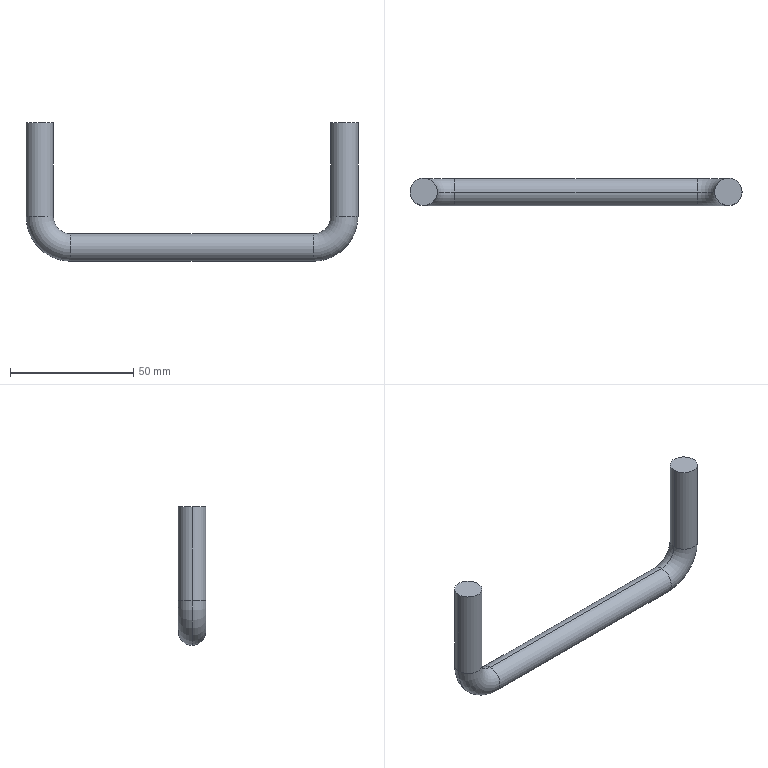Part | NX | features BREP 1 | 1 solid | 12 faces | box 134.938 x 11.113 x 56.356 mm | volume 20806 mm3 | cylinder 6 | torus 4 | plane 2 | commonest cylinder face diameters 11.113 x6
STEP:
#1=CARTESIAN_POINT('',(-56.356,0.,0.));
#2=VERTEX_POINT('',#1);
#3=CARTESIAN_POINT('',(-67.469,0.,0.));
#4=VERTEX_POINT('',#3);
#5=CARTESIAN_POINT('',(-61.913,0.,0.));
#6=DIRECTION('',(0.,0.,-1.));
#7=DIRECTION('',(1.,0.,0.));
#8=AXIS2_PLACEMENT_3D('',#5,#6,#7);
#9=CIRCLE('',#8,5.556);
#10=EDGE_CURVE('',#2,#4,#9,.T.);
#11=ORIENTED_EDGE('',*,*,#10,.F.);
#12=CARTESIAN_POINT('',(-61.913,0.,0.));
#13=DIRECTION('',(0.,0.,-1.));
#14=DIRECTION('',(-1.,0.,0.));
#15=AXIS2_PLACEMENT_3D('',#12,#13,#14);
#16=CIRCLE('',#15,5.556);
#17=EDGE_CURVE('',#4,#2,#16,.T.);
#18=ORIENTED_EDGE('',*,*,#17,.F.);
#19=EDGE_LOOP('',(#11,#18));
#20=FACE_BOUND('',#19,.T.);
#21=CARTESIAN_POINT('',(-61.913,0.,0.));
#22=DIRECTION('',(0.,0.,-1.));
#23=DIRECTION('',(0.,-1.,0.));
#24=AXIS2_PLACEMENT_3D('',#21,#22,#23);
#25=PLANE('',#24);
#26=ADVANCED_FACE('',(#20),#25,.F.);
#27=CARTESIAN_POINT('',(-56.356,0.,-38.1));
#28=VERTEX_POINT('',#27);
#29=CARTESIAN_POINT('',(-56.356,0.,0.));
#30=DIRECTION('',(0.,0.,-1.));
#31=VECTOR('',#30,1000.);
#32=LINE('',#29,#31);
#33=EDGE_CURVE('',#28,#2,#32,.F.);
#34=ORIENTED_EDGE('',*,*,#33,.F.);
#35=CARTESIAN_POINT('',(-67.469,0.,-38.1));
#36=VERTEX_POINT('',#35);
#37=CARTESIAN_POINT('',(-61.913,0.,-38.1));
#38=DIRECTION('',(0.,0.,-1.));
#39=DIRECTION('',(-1.,0.,0.));
#40=AXIS2_PLACEMENT_3D('',#37,#38,#39);
#41=CIRCLE('',#40,5.556);
#42=EDGE_CURVE('',#36,#28,#41,.T.);
#43=ORIENTED_EDGE('',*,*,#42,.F.);
#44=CARTESIAN_POINT('',(-67.469,0.,0.));
#45=DIRECTION('',(0.,0.,-1.));
#46=VECTOR('',#45,1000.);
#47=LINE('',#44,#46);
#48=EDGE_CURVE('',#36,#4,#47,.F.);
#49=ORIENTED_EDGE('',*,*,#48,.T.);
#50=ORIENTED_EDGE('',*,*,#17,.T.);
#51=EDGE_LOOP('',(#34,#43,#49,#50));
#52=FACE_BOUND('',#51,.T.);
#53=CARTESIAN_POINT('',(-61.913,0.,0.));
#54=DIRECTION('',(0.,0.,-1.));
#55=DIRECTION('',(-1.,0.,0.));
#56=AXIS2_PLACEMENT_3D('',#53,#54,#55);
#57=CYLINDRICAL_SURFACE('',#56,5.556);
#58=ADVANCED_FACE('',(#52),#57,.T.);
#59=ORIENTED_EDGE('',*,*,#48,.F.);
#60=CARTESIAN_POINT('',(-61.913,0.,-38.1));
#61=DIRECTION('',(0.,0.,-1.));
#62=DIRECTION('',(1.,0.,0.));
#63=AXIS2_PLACEMENT_3D('',#60,#61,#62);
#64=CIRCLE('',#63,5.556);
#65=EDGE_CURVE('',#28,#36,#64,.T.);
#66=ORIENTED_EDGE('',*,*,#65,.F.);
#67=ORIENTED_EDGE('',*,*,#33,.T.);
#68=ORIENTED_EDGE('',*,*,#10,.T.);
#69=EDGE_LOOP('',(#59,#66,#67,#68));
#70=FACE_BOUND('',#69,.T.);
#71=CARTESIAN_POINT('',(-61.913,0.,0.));
#72=DIRECTION('',(0.,0.,-1.));
#73=DIRECTION('',(-1.,0.,0.));
#74=AXIS2_PLACEMENT_3D('',#71,#72,#73);
#75=CYLINDRICAL_SURFACE('',#74,5.556);
#76=ADVANCED_FACE('',(#70),#75,.T.);
#77=CARTESIAN_POINT('',(-49.212,0.,-56.356));
#78=VERTEX_POINT('',#77);
#79=CARTESIAN_POINT('',(-49.212,0.,-38.1));
#80=DIRECTION('',(0.,-1.,0.));
#81=DIRECTION('',(-1.,0.,0.));
#82=AXIS2_PLACEMENT_3D('',#79,#80,#81);
#83=CIRCLE('',#82,18.256);
#84=EDGE_CURVE('',#36,#78,#83,.T.);
#85=ORIENTED_EDGE('',*,*,#84,.T.);
#86=CARTESIAN_POINT('',(-49.212,0.,-45.244));
#87=VERTEX_POINT('',#86);
#88=CARTESIAN_POINT('',(-49.212,0.,-50.8));
#89=DIRECTION('',(1.,0.,0.));
#90=DIRECTION('',(0.,0.,1.));
#91=AXIS2_PLACEMENT_3D('',#88,#89,#90);
#92=CIRCLE('',#91,5.556);
#93=EDGE_CURVE('',#87,#78,#92,.T.);
#94=ORIENTED_EDGE('',*,*,#93,.F.);
#95=CARTESIAN_POINT('',(-49.212,0.,-38.1));
#96=DIRECTION('',(0.,-1.,0.));
#97=DIRECTION('',(-1.,0.,0.));
#98=AXIS2_PLACEMENT_3D('',#95,#96,#97);
#99=CIRCLE('',#98,7.144);
#100=EDGE_CURVE('',#28,#87,#99,.T.);
#101=ORIENTED_EDGE('',*,*,#100,.F.);
#102=ORIENTED_EDGE('',*,*,#65,.T.);
#103=EDGE_LOOP('',(#85,#94,#101,#102));
#104=FACE_BOUND('',#103,.T.);
#105=CARTESIAN_POINT('',(-49.212,0.,-38.1));
#106=DIRECTION('',(0.,-1.,0.));
#107=DIRECTION('',(1.,0.,0.));
#108=AXIS2_PLACEMENT_3D('',#105,#106,#107);
#109=TOROIDAL_SURFACE('',#108,12.7,5.556);
#110=ADVANCED_FACE('',(#104),#109,.T.);
#111=ORIENTED_EDGE('',*,*,#100,.T.);
#112=CARTESIAN_POINT('',(-49.212,0.,-50.8));
#113=DIRECTION('',(1.,0.,0.));
#114=DIRECTION('',(0.,0.,-1.));
#115=AXIS2_PLACEMENT_3D('',#112,#113,#114);
#116=CIRCLE('',#115,5.556);
#117=EDGE_CURVE('',#78,#87,#116,.T.);
#118=ORIENTED_EDGE('',*,*,#117,.F.);
#119=ORIENTED_EDGE('',*,*,#84,.F.);
#120=ORIENTED_EDGE('',*,*,#42,.T.);
#121=EDGE_LOOP('',(#111,#118,#119,#120));
#122=FACE_BOUND('',#121,.T.);
#123=CARTESIAN_POINT('',(-49.212,0.,-38.1));
#124=DIRECTION('',(0.,-1.,0.));
#125=DIRECTION('',(1.,0.,0.));
#126=AXIS2_PLACEMENT_3D('',#123,#124,#125);
#127=TOROIDAL_SURFACE('',#126,12.7,5.556);
#128=ADVANCED_FACE('',(#122),#127,.T.);
#129=CARTESIAN_POINT('',(49.212,0.,-45.244));
#130=VERTEX_POINT('',#129);
#131=CARTESIAN_POINT('',(-49.212,0.,-45.244));
#132=DIRECTION('',(1.,0.,0.));
#133=VECTOR('',#132,1000.);
#134=LINE('',#131,#133);
#135=EDGE_CURVE('',#130,#87,#134,.F.);
#136=ORIENTED_EDGE('',*,*,#135,.F.);
#137=CARTESIAN_POINT('',(49.212,0.,-56.356));
#138=VERTEX_POINT('',#137);
#139=CARTESIAN_POINT('',(49.212,0.,-50.8));
#140=DIRECTION('',(1.,0.,0.));
#141=DIRECTION('',(0.,0.,-1.));
#142=AXIS2_PLACEMENT_3D('',#139,#140,#141);
#143=CIRCLE('',#142,5.556);
#144=EDGE_CURVE('',#138,#130,#143,.T.);
#145=ORIENTED_EDGE('',*,*,#144,.F.);
#146=CARTESIAN_POINT('',(-49.212,0.,-56.356));
#147=DIRECTION('',(1.,0.,0.));
#148=VECTOR('',#147,1000.);
#149=LINE('',#146,#148);
#150=EDGE_CURVE('',#138,#78,#149,.F.);
#151=ORIENTED_EDGE('',*,*,#150,.T.);
#152=ORIENTED_EDGE('',*,*,#117,.T.);
#153=EDGE_LOOP('',(#136,#145,#151,#152));
#154=FACE_BOUND('',#153,.T.);
#155=CARTESIAN_POINT('',(-49.212,0.,-50.8));
#156=DIRECTION('',(1.,0.,0.));
#157=DIRECTION('',(0.,0.,-1.));
#158=AXIS2_PLACEMENT_3D('',#155,#156,#157);
#159=CYLINDRICAL_SURFACE('',#158,5.556);
#160=ADVANCED_FACE('',(#154),#159,.T.);
#161=ORIENTED_EDGE('',*,*,#150,.F.);
#162=CARTESIAN_POINT('',(49.212,0.,-50.8));
#163=DIRECTION('',(1.,0.,0.));
#164=DIRECTION('',(0.,0.,1.));
#165=AXIS2_PLACEMENT_3D('',#162,#163,#164);
#166=CIRCLE('',#165,5.556);
#167=EDGE_CURVE('',#130,#138,#166,.T.);
#168=ORIENTED_EDGE('',*,*,#167,.F.);
#169=ORIENTED_EDGE('',*,*,#135,.T.);
#170=ORIENTED_EDGE('',*,*,#93,.T.);
#171=EDGE_LOOP('',(#161,#168,#169,#170));
#172=FACE_BOUND('',#171,.T.);
#173=CARTESIAN_POINT('',(-49.212,0.,-50.8));
#174=DIRECTION('',(1.,0.,0.));
#175=DIRECTION('',(0.,0.,-1.));
#176=AXIS2_PLACEMENT_3D('',#173,#174,#175);
#177=CYLINDRICAL_SURFACE('',#176,5.556);
#178=ADVANCED_FACE('',(#172),#177,.T.);
#179=CARTESIAN_POINT('',(67.469,0.,-38.1));
#180=VERTEX_POINT('',#179);
#181=CARTESIAN_POINT('',(49.212,0.,-38.1));
#182=DIRECTION('',(0.,-1.,0.));
#183=DIRECTION('',(0.,0.,-1.));
#184=AXIS2_PLACEMENT_3D('',#181,#182,#183);
#185=CIRCLE('',#184,18.256);
#186=EDGE_CURVE('',#138,#180,#185,.T.);
#187=ORIENTED_EDGE('',*,*,#186,.T.);
#188=CARTESIAN_POINT('',(56.356,0.,-38.1));
#189=VERTEX_POINT('',#188);
#190=CARTESIAN_POINT('',(61.913,0.,-38.1));
#191=DIRECTION('',(0.,0.,1.));
#192=DIRECTION('',(-1.,0.,0.));
#193=AXIS2_PLACEMENT_3D('',#190,#191,#192);
#194=CIRCLE('',#193,5.556);
#195=EDGE_CURVE('',#189,#180,#194,.T.);
#196=ORIENTED_EDGE('',*,*,#195,.F.);
#197=CARTESIAN_POINT('',(49.212,0.,-38.1));
#198=DIRECTION('',(0.,-1.,0.));
#199=DIRECTION('',(0.,0.,-1.));
#200=AXIS2_PLACEMENT_3D('',#197,#198,#199);
#201=CIRCLE('',#200,7.144);
#202=EDGE_CURVE('',#130,#189,#201,.T.);
#203=ORIENTED_EDGE('',*,*,#202,.F.);
#204=ORIENTED_EDGE('',*,*,#167,.T.);
#205=EDGE_LOOP('',(#187,#196,#203,#204));
#206=FACE_BOUND('',#205,.T.);
#207=CARTESIAN_POINT('',(49.212,0.,-38.1));
#208=DIRECTION('',(0.,-1.,0.));
#209=DIRECTION('',(0.,0.,1.));
#210=AXIS2_PLACEMENT_3D('',#207,#208,#209);
#211=TOROIDAL_SURFACE('',#210,12.7,5.556);
#212=ADVANCED_FACE('',(#206),#211,.T.);
#213=ORIENTED_EDGE('',*,*,#202,.T.);
#214=CARTESIAN_POINT('',(61.913,0.,-38.1));
#215=DIRECTION('',(0.,0.,1.));
#216=DIRECTION('',(1.,0.,0.));
#217=AXIS2_PLACEMENT_3D('',#214,#215,#216);
#218=CIRCLE('',#217,5.556);
#219=EDGE_CURVE('',#180,#189,#218,.T.);
#220=ORIENTED_EDGE('',*,*,#219,.F.);
#221=ORIENTED_EDGE('',*,*,#186,.F.);
#222=ORIENTED_EDGE('',*,*,#144,.T.);
#223=EDGE_LOOP('',(#213,#220,#221,#222));
#224=FACE_BOUND('',#223,.T.);
#225=CARTESIAN_POINT('',(49.212,0.,-38.1));
#226=DIRECTION('',(0.,-1.,0.));
#227=DIRECTION('',(0.,0.,1.));
#228=AXIS2_PLACEMENT_3D('',#225,#226,#227);
#229=TOROIDAL_SURFACE('',#228,12.7,5.556);
#230=ADVANCED_FACE('',(#224),#229,.T.);
#231=CARTESIAN_POINT('',(56.356,0.,0.));
#232=VERTEX_POINT('',#231);
#233=CARTESIAN_POINT('',(56.356,0.,-38.1));
#234=DIRECTION('',(0.,0.,1.));
#235=VECTOR('',#234,1000.);
#236=LINE('',#233,#235);
#237=EDGE_CURVE('',#189,#232,#236,.T.);
#238=ORIENTED_EDGE('',*,*,#237,.T.);
#239=CARTESIAN_POINT('',(67.469,0.,0.));
#240=VERTEX_POINT('',#239);
#241=CARTESIAN_POINT('',(61.913,0.,0.));
#242=DIRECTION('',(0.,0.,1.));
#243=DIRECTION('',(1.,0.,0.));
#244=AXIS2_PLACEMENT_3D('',#241,#242,#243);
#245=CIRCLE('',#244,5.556);
#246=EDGE_CURVE('',#240,#232,#245,.T.);
#247=ORIENTED_EDGE('',*,*,#246,.F.);
#248=CARTESIAN_POINT('',(67.469,0.,-38.1));
#249=DIRECTION('',(0.,0.,1.));
#250=VECTOR('',#249,1000.);
#251=LINE('',#248,#250);
#252=EDGE_CURVE('',#180,#240,#251,.T.);
#253=ORIENTED_EDGE('',*,*,#252,.F.);
#254=ORIENTED_EDGE('',*,*,#219,.T.);
#255=EDGE_LOOP('',(#238,#247,#253,#254));
#256=FACE_BOUND('',#255,.T.);
#257=CARTESIAN_POINT('',(61.913,0.,-38.1));
#258=DIRECTION('',(0.,0.,1.));
#259=DIRECTION('',(1.,0.,0.));
#260=AXIS2_PLACEMENT_3D('',#257,#258,#259);
#261=CYLINDRICAL_SURFACE('',#260,5.556);
#262=ADVANCED_FACE('',(#256),#261,.T.);
#263=ORIENTED_EDGE('',*,*,#252,.T.);
#264=CARTESIAN_POINT('',(61.913,0.,0.));
#265=DIRECTION('',(0.,0.,1.));
#266=DIRECTION('',(-1.,0.,0.));
#267=AXIS2_PLACEMENT_3D('',#264,#265,#266);
#268=CIRCLE('',#267,5.556);
#269=EDGE_CURVE('',#232,#240,#268,.T.);
#270=ORIENTED_EDGE('',*,*,#269,.F.);
#271=ORIENTED_EDGE('',*,*,#237,.F.);
#272=ORIENTED_EDGE('',*,*,#195,.T.);
#273=EDGE_LOOP('',(#263,#270,#271,#272));
#274=FACE_BOUND('',#273,.T.);
#275=CARTESIAN_POINT('',(61.913,0.,-38.1));
#276=DIRECTION('',(0.,0.,1.));
#277=DIRECTION('',(1.,0.,0.));
#278=AXIS2_PLACEMENT_3D('',#275,#276,#277);
#279=CYLINDRICAL_SURFACE('',#278,5.556);
#280=ADVANCED_FACE('',(#274),#279,.T.);
#281=ORIENTED_EDGE('',*,*,#269,.T.);
#282=ORIENTED_EDGE('',*,*,#246,.T.);
#283=EDGE_LOOP('',(#281,#282));
#284=FACE_BOUND('',#283,.T.);
#285=CARTESIAN_POINT('',(61.913,0.,0.));
#286=DIRECTION('',(0.,0.,1.));
#287=DIRECTION('',(1.,0.,0.));
#288=AXIS2_PLACEMENT_3D('',#285,#286,#287);
#289=PLANE('',#288);
#290=ADVANCED_FACE('',(#284),#289,.T.);
#291=CLOSED_SHELL('',(#26,#58,#76,#110,#128,#160,#178,#212,#230,#262,#280,#290));
#292=MANIFOLD_SOLID_BREP('',#291);
#293=(LENGTH_UNIT()NAMED_UNIT(*)SI_UNIT(.MILLI.,.METRE.));
#294=UNCERTAINTY_MEASURE_WITH_UNIT(LENGTH_MEASURE(0.00001),#293,'','');
#295=(NAMED_UNIT(*)PLANE_ANGLE_UNIT()SI_UNIT($,.RADIAN.));
#296=(NAMED_UNIT(*)SI_UNIT($,.STERADIAN.)SOLID_ANGLE_UNIT());
#297=(GEOMETRIC_REPRESENTATION_CONTEXT(3)GLOBAL_UNCERTAINTY_ASSIGNED_CONTEXT((#294))GLOBAL_UNIT_ASSIGNED_CONTEXT((#293,#295,#296))REPRESENTATION_CONTEXT('',''));
#298=ADVANCED_BREP_SHAPE_REPRESENTATION('',(#292),#297);